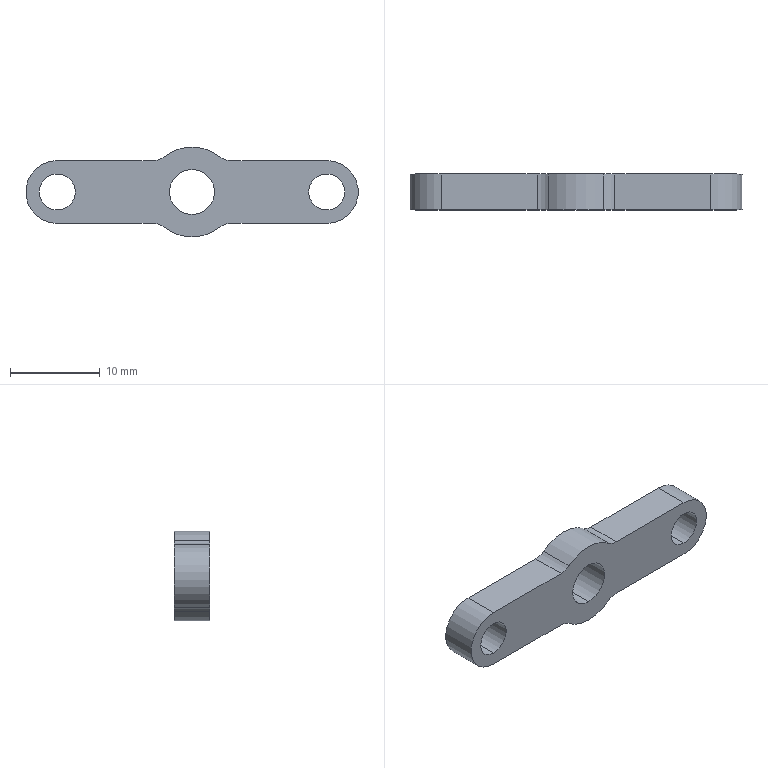Part | SolidWorks | features Extrusion 1, Scale 1 | 1 solid | 21 faces | box 37 x 4 x 10 mm | volume 874.953 mm3 | cylinder 15 | plane 6 | commonest cylinder face diameters 4 x8 10 x3 5 x2 7 x2
STEP:
#1=CARTESIAN_POINT('',(-15.,4.,-2.));
#2=VERTEX_POINT('',#1);
#3=CARTESIAN_POINT('',(-15.,4.,2.));
#4=VERTEX_POINT('',#3);
#5=CARTESIAN_POINT('',(-15.,4.,0.));
#6=DIRECTION('',(0.,1.,0.));
#7=DIRECTION('',(0.,0.,-1.));
#8=AXIS2_PLACEMENT_3D('',#5,#6,#7);
#9=CIRCLE('',#8,2.);
#10=EDGE_CURVE('',#2,#4,#9,.T.);
#11=ORIENTED_EDGE('',*,*,#10,.T.);
#12=CARTESIAN_POINT('',(-15.,0.,2.));
#13=VERTEX_POINT('',#12);
#14=CARTESIAN_POINT('',(-15.,4.,2.));
#15=DIRECTION('',(0.,-1.,0.));
#16=VECTOR('',#15,1000.);
#17=LINE('',#14,#16);
#18=EDGE_CURVE('',#4,#13,#17,.T.);
#19=ORIENTED_EDGE('',*,*,#18,.T.);
#20=CARTESIAN_POINT('',(-15.,0.,-2.));
#21=VERTEX_POINT('',#20);
#22=CARTESIAN_POINT('',(-15.,0.,0.));
#23=DIRECTION('',(0.,1.,0.));
#24=DIRECTION('',(0.,0.,-1.));
#25=AXIS2_PLACEMENT_3D('',#22,#23,#24);
#26=CIRCLE('',#25,2.);
#27=EDGE_CURVE('',#21,#13,#26,.T.);
#28=ORIENTED_EDGE('',*,*,#27,.F.);
#29=CARTESIAN_POINT('',(-15.,4.,-2.));
#30=DIRECTION('',(0.,-1.,0.));
#31=VECTOR('',#30,1000.);
#32=LINE('',#29,#31);
#33=EDGE_CURVE('',#2,#21,#32,.T.);
#34=ORIENTED_EDGE('',*,*,#33,.F.);
#35=EDGE_LOOP('',(#11,#19,#28,#34));
#36=FACE_OUTER_BOUND('',#35,.T.);
#37=CARTESIAN_POINT('',(-15.,4.,0.));
#38=DIRECTION('',(0.,-1.,0.));
#39=DIRECTION('',(0.,0.,-1.));
#40=AXIS2_PLACEMENT_3D('',#37,#38,#39);
#41=CYLINDRICAL_SURFACE('',#40,2.);
#42=ADVANCED_FACE('',(#36),#41,.F.);
#43=CARTESIAN_POINT('',(15.,4.,-2.));
#44=VERTEX_POINT('',#43);
#45=CARTESIAN_POINT('',(15.,4.,2.));
#46=VERTEX_POINT('',#45);
#47=CARTESIAN_POINT('',(15.,4.,0.));
#48=DIRECTION('',(0.,1.,0.));
#49=DIRECTION('',(0.,0.,1.));
#50=AXIS2_PLACEMENT_3D('',#47,#48,#49);
#51=CIRCLE('',#50,2.);
#52=EDGE_CURVE('',#44,#46,#51,.T.);
#53=ORIENTED_EDGE('',*,*,#52,.T.);
#54=CARTESIAN_POINT('',(15.,0.,2.));
#55=VERTEX_POINT('',#54);
#56=CARTESIAN_POINT('',(15.,4.,2.));
#57=DIRECTION('',(0.,-1.,0.));
#58=VECTOR('',#57,1000.);
#59=LINE('',#56,#58);
#60=EDGE_CURVE('',#46,#55,#59,.T.);
#61=ORIENTED_EDGE('',*,*,#60,.T.);
#62=CARTESIAN_POINT('',(15.,0.,-2.));
#63=VERTEX_POINT('',#62);
#64=CARTESIAN_POINT('',(15.,0.,0.));
#65=DIRECTION('',(0.,1.,0.));
#66=DIRECTION('',(0.,0.,1.));
#67=AXIS2_PLACEMENT_3D('',#64,#65,#66);
#68=CIRCLE('',#67,2.);
#69=EDGE_CURVE('',#63,#55,#68,.T.);
#70=ORIENTED_EDGE('',*,*,#69,.F.);
#71=CARTESIAN_POINT('',(15.,4.,-2.));
#72=DIRECTION('',(0.,-1.,0.));
#73=VECTOR('',#72,1000.);
#74=LINE('',#71,#73);
#75=EDGE_CURVE('',#44,#63,#74,.T.);
#76=ORIENTED_EDGE('',*,*,#75,.F.);
#77=EDGE_LOOP('',(#53,#61,#70,#76));
#78=FACE_OUTER_BOUND('',#77,.T.);
#79=CARTESIAN_POINT('',(15.,4.,0.));
#80=DIRECTION('',(0.,-1.,0.));
#81=DIRECTION('',(0.,0.,-1.));
#82=AXIS2_PLACEMENT_3D('',#79,#80,#81);
#83=CYLINDRICAL_SURFACE('',#82,2.);
#84=ADVANCED_FACE('',(#78),#83,.F.);
#85=CARTESIAN_POINT('',(0.,4.,-2.5));
#86=VERTEX_POINT('',#85);
#87=CARTESIAN_POINT('',(0.,4.,2.5));
#88=VERTEX_POINT('',#87);
#89=CARTESIAN_POINT('',(0.,4.,0.));
#90=DIRECTION('',(0.,1.,0.));
#91=DIRECTION('',(0.,0.,1.));
#92=AXIS2_PLACEMENT_3D('',#89,#90,#91);
#93=CIRCLE('',#92,2.5);
#94=EDGE_CURVE('',#86,#88,#93,.T.);
#95=ORIENTED_EDGE('',*,*,#94,.T.);
#96=CARTESIAN_POINT('',(0.,0.,2.5));
#97=VERTEX_POINT('',#96);
#98=CARTESIAN_POINT('',(0.,4.,2.5));
#99=DIRECTION('',(0.,-1.,0.));
#100=VECTOR('',#99,1000.);
#101=LINE('',#98,#100);
#102=EDGE_CURVE('',#88,#97,#101,.T.);
#103=ORIENTED_EDGE('',*,*,#102,.T.);
#104=CARTESIAN_POINT('',(0.,0.,-2.5));
#105=VERTEX_POINT('',#104);
#106=CARTESIAN_POINT('',(0.,0.,0.));
#107=DIRECTION('',(0.,1.,0.));
#108=DIRECTION('',(0.,0.,1.));
#109=AXIS2_PLACEMENT_3D('',#106,#107,#108);
#110=CIRCLE('',#109,2.5);
#111=EDGE_CURVE('',#105,#97,#110,.T.);
#112=ORIENTED_EDGE('',*,*,#111,.F.);
#113=CARTESIAN_POINT('',(0.,4.,-2.5));
#114=DIRECTION('',(0.,-1.,0.));
#115=VECTOR('',#114,1000.);
#116=LINE('',#113,#115);
#117=EDGE_CURVE('',#86,#105,#116,.T.);
#118=ORIENTED_EDGE('',*,*,#117,.F.);
#119=EDGE_LOOP('',(#95,#103,#112,#118));
#120=FACE_OUTER_BOUND('',#119,.T.);
#121=CARTESIAN_POINT('',(0.,4.,0.));
#122=DIRECTION('',(0.,-1.,0.));
#123=DIRECTION('',(0.,0.,-1.));
#124=AXIS2_PLACEMENT_3D('',#121,#122,#123);
#125=CYLINDRICAL_SURFACE('',#124,2.5);
#126=ADVANCED_FACE('',(#120),#125,.F.);
#127=CARTESIAN_POINT('',(0.,4.,-5.));
#128=VERTEX_POINT('',#127);
#129=CARTESIAN_POINT('',(-3.093,4.,-3.929));
#130=VERTEX_POINT('',#129);
#131=CARTESIAN_POINT('',(0.,4.,0.));
#132=DIRECTION('',(0.,1.,0.));
#133=DIRECTION('',(0.,0.,1.));
#134=AXIS2_PLACEMENT_3D('',#131,#132,#133);
#135=CIRCLE('',#134,5.);
#136=EDGE_CURVE('',#128,#130,#135,.T.);
#137=ORIENTED_EDGE('',*,*,#136,.F.);
#138=CARTESIAN_POINT('',(0.,0.,-5.));
#139=VERTEX_POINT('',#138);
#140=CARTESIAN_POINT('',(0.,4.,-5.));
#141=DIRECTION('',(0.,-1.,0.));
#142=VECTOR('',#141,1000.);
#143=LINE('',#140,#142);
#144=EDGE_CURVE('',#128,#139,#143,.T.);
#145=ORIENTED_EDGE('',*,*,#144,.T.);
#146=CARTESIAN_POINT('',(-3.093,0.,-3.929));
#147=VERTEX_POINT('',#146);
#148=CARTESIAN_POINT('',(0.,0.,0.));
#149=DIRECTION('',(0.,1.,0.));
#150=DIRECTION('',(0.,0.,1.));
#151=AXIS2_PLACEMENT_3D('',#148,#149,#150);
#152=CIRCLE('',#151,5.);
#153=EDGE_CURVE('',#139,#147,#152,.T.);
#154=ORIENTED_EDGE('',*,*,#153,.T.);
#155=CARTESIAN_POINT('',(-3.093,4.,-3.929));
#156=DIRECTION('',(0.,-1.,0.));
#157=VECTOR('',#156,1000.);
#158=LINE('',#155,#157);
#159=EDGE_CURVE('',#130,#147,#158,.T.);
#160=ORIENTED_EDGE('',*,*,#159,.F.);
#161=EDGE_LOOP('',(#137,#145,#154,#160));
#162=FACE_OUTER_BOUND('',#161,.T.);
#163=CARTESIAN_POINT('',(0.,4.,0.));
#164=DIRECTION('',(0.,-1.,0.));
#165=DIRECTION('',(0.,0.,-1.));
#166=AXIS2_PLACEMENT_3D('',#163,#164,#165);
#167=CYLINDRICAL_SURFACE('',#166,5.);
#168=ADVANCED_FACE('',(#162),#167,.T.);
#169=ORIENTED_EDGE('',*,*,#52,.F.);
#170=CARTESIAN_POINT('',(15.,4.,0.));
#171=DIRECTION('',(0.,1.,0.));
#172=DIRECTION('',(0.,0.,1.));
#173=AXIS2_PLACEMENT_3D('',#170,#171,#172);
#174=CIRCLE('',#173,2.);
#175=EDGE_CURVE('',#46,#44,#174,.T.);
#176=ORIENTED_EDGE('',*,*,#175,.F.);
#177=EDGE_LOOP('',(#169,#176));
#178=FACE_BOUND('',#177,.T.);
#179=CARTESIAN_POINT('',(3.093,4.,3.929));
#180=VERTEX_POINT('',#179);
#181=CARTESIAN_POINT('',(4.33,4.,3.5));
#182=VERTEX_POINT('',#181);
#183=CARTESIAN_POINT('',(4.33,4.,5.5));
#184=DIRECTION('',(0.,-1.,0.));
#185=DIRECTION('',(0.,0.,1.));
#186=AXIS2_PLACEMENT_3D('',#183,#184,#185);
#187=CIRCLE('',#186,2.);
#188=EDGE_CURVE('',#180,#182,#187,.T.);
#189=ORIENTED_EDGE('',*,*,#188,.T.);
#190=CARTESIAN_POINT('',(15.,4.,3.5));
#191=VERTEX_POINT('',#190);
#192=CARTESIAN_POINT('',(15.,4.,3.5));
#193=DIRECTION('',(1.,0.,0.));
#194=VECTOR('',#193,1000.);
#195=LINE('',#192,#194);
#196=EDGE_CURVE('',#182,#191,#195,.T.);
#197=ORIENTED_EDGE('',*,*,#196,.T.);
#198=CARTESIAN_POINT('',(15.,4.,-3.5));
#199=VERTEX_POINT('',#198);
#200=CARTESIAN_POINT('',(15.,4.,0.));
#201=DIRECTION('',(0.,1.,0.));
#202=DIRECTION('',(0.,0.,1.));
#203=AXIS2_PLACEMENT_3D('',#200,#201,#202);
#204=CIRCLE('',#203,3.5);
#205=EDGE_CURVE('',#191,#199,#204,.T.);
#206=ORIENTED_EDGE('',*,*,#205,.T.);
#207=CARTESIAN_POINT('',(4.33,4.,-3.5));
#208=VERTEX_POINT('',#207);
#209=CARTESIAN_POINT('',(15.,4.,-3.5));
#210=DIRECTION('',(-1.,0.,0.));
#211=VECTOR('',#210,1000.);
#212=LINE('',#209,#211);
#213=EDGE_CURVE('',#199,#208,#212,.T.);
#214=ORIENTED_EDGE('',*,*,#213,.T.);
#215=CARTESIAN_POINT('',(3.093,4.,-3.929));
#216=VERTEX_POINT('',#215);
#217=CARTESIAN_POINT('',(4.33,4.,-5.5));
#218=DIRECTION('',(0.,-1.,0.));
#219=DIRECTION('',(0.,0.,-1.));
#220=AXIS2_PLACEMENT_3D('',#217,#218,#219);
#221=CIRCLE('',#220,2.);
#222=EDGE_CURVE('',#208,#216,#221,.T.);
#223=ORIENTED_EDGE('',*,*,#222,.T.);
#224=CARTESIAN_POINT('',(0.,4.,0.));
#225=DIRECTION('',(0.,1.,0.));
#226=DIRECTION('',(0.,0.,1.));
#227=AXIS2_PLACEMENT_3D('',#224,#225,#226);
#228=CIRCLE('',#227,5.);
#229=EDGE_CURVE('',#216,#128,#228,.T.);
#230=ORIENTED_EDGE('',*,*,#229,.T.);
#231=ORIENTED_EDGE('',*,*,#136,.T.);
#232=CARTESIAN_POINT('',(-4.33,4.,-3.5));
#233=VERTEX_POINT('',#232);
#234=CARTESIAN_POINT('',(-4.33,4.,-5.5));
#235=DIRECTION('',(0.,-1.,0.));
#236=DIRECTION('',(0.,0.,1.));
#237=AXIS2_PLACEMENT_3D('',#234,#235,#236);
#238=CIRCLE('',#237,2.);
#239=EDGE_CURVE('',#130,#233,#238,.T.);
#240=ORIENTED_EDGE('',*,*,#239,.T.);
#241=CARTESIAN_POINT('',(-15.,4.,-3.5));
#242=VERTEX_POINT('',#241);
#243=CARTESIAN_POINT('',(-15.,4.,-3.5));
#244=DIRECTION('',(-1.,0.,0.));
#245=VECTOR('',#244,1000.);
#246=LINE('',#243,#245);
#247=EDGE_CURVE('',#233,#242,#246,.T.);
#248=ORIENTED_EDGE('',*,*,#247,.T.);
#249=CARTESIAN_POINT('',(-15.,4.,3.5));
#250=VERTEX_POINT('',#249);
#251=CARTESIAN_POINT('',(-15.,4.,0.));
#252=DIRECTION('',(0.,1.,0.));
#253=DIRECTION('',(0.,0.,-1.));
#254=AXIS2_PLACEMENT_3D('',#251,#252,#253);
#255=CIRCLE('',#254,3.5);
#256=EDGE_CURVE('',#242,#250,#255,.T.);
#257=ORIENTED_EDGE('',*,*,#256,.T.);
#258=CARTESIAN_POINT('',(-4.33,4.,3.5));
#259=VERTEX_POINT('',#258);
#260=CARTESIAN_POINT('',(-15.,4.,3.5));
#261=DIRECTION('',(1.,0.,0.));
#262=VECTOR('',#261,1000.);
#263=LINE('',#260,#262);
#264=EDGE_CURVE('',#250,#259,#263,.T.);
#265=ORIENTED_EDGE('',*,*,#264,.T.);
#266=CARTESIAN_POINT('',(-3.093,4.,3.929));
#267=VERTEX_POINT('',#266);
#268=CARTESIAN_POINT('',(-4.33,4.,5.5));
#269=DIRECTION('',(0.,-1.,0.));
#270=DIRECTION('',(0.,0.,-1.));
#271=AXIS2_PLACEMENT_3D('',#268,#269,#270);
#272=CIRCLE('',#271,2.);
#273=EDGE_CURVE('',#259,#267,#272,.T.);
#274=ORIENTED_EDGE('',*,*,#273,.T.);
#275=CARTESIAN_POINT('',(0.,4.,0.));
#276=DIRECTION('',(0.,1.,0.));
#277=DIRECTION('',(0.,0.,1.));
#278=AXIS2_PLACEMENT_3D('',#275,#276,#277);
#279=CIRCLE('',#278,5.);
#280=EDGE_CURVE('',#267,#180,#279,.T.);
#281=ORIENTED_EDGE('',*,*,#280,.T.);
#282=EDGE_LOOP('',(#189,#197,#206,#214,#223,#230,#231,#240,#248,#257,#265,#274,#281));
#283=FACE_OUTER_BOUND('',#282,.T.);
#284=ORIENTED_EDGE('',*,*,#94,.F.);
#285=CARTESIAN_POINT('',(0.,4.,0.));
#286=DIRECTION('',(0.,1.,0.));
#287=DIRECTION('',(0.,0.,1.));
#288=AXIS2_PLACEMENT_3D('',#285,#286,#287);
#289=CIRCLE('',#288,2.5);
#290=EDGE_CURVE('',#88,#86,#289,.T.);
#291=ORIENTED_EDGE('',*,*,#290,.F.);
#292=EDGE_LOOP('',(#284,#291));
#293=FACE_BOUND('',#292,.T.);
#294=ORIENTED_EDGE('',*,*,#10,.F.);
#295=CARTESIAN_POINT('',(-15.,4.,0.));
#296=DIRECTION('',(0.,1.,0.));
#297=DIRECTION('',(0.,0.,-1.));
#298=AXIS2_PLACEMENT_3D('',#295,#296,#297);
#299=CIRCLE('',#298,2.);
#300=EDGE_CURVE('',#4,#2,#299,.T.);
#301=ORIENTED_EDGE('',*,*,#300,.F.);
#302=EDGE_LOOP('',(#294,#301));
#303=FACE_BOUND('',#302,.T.);
#304=CARTESIAN_POINT('',(4.33,4.,5.5));
#305=DIRECTION('',(0.,1.,0.));
#306=DIRECTION('',(0.,0.,1.));
#307=AXIS2_PLACEMENT_3D('',#304,#305,#306);
#308=PLANE('',#307);
#309=ADVANCED_FACE('',(#178,#283,#293,#303),#308,.T.);
#310=CARTESIAN_POINT('',(3.093,0.,3.929));
#311=VERTEX_POINT('',#310);
#312=CARTESIAN_POINT('',(4.33,0.,3.5));
#313=VERTEX_POINT('',#312);
#314=CARTESIAN_POINT('',(4.33,0.,5.5));
#315=DIRECTION('',(0.,-1.,0.));
#316=DIRECTION('',(0.,0.,1.));
#317=AXIS2_PLACEMENT_3D('',#314,#315,#316);
#318=CIRCLE('',#317,2.);
#319=EDGE_CURVE('',#311,#313,#318,.T.);
#320=ORIENTED_EDGE('',*,*,#319,.F.);
#321=CARTESIAN_POINT('',(-3.093,0.,3.929));
#322=VERTEX_POINT('',#321);
#323=CARTESIAN_POINT('',(0.,0.,0.));
#324=DIRECTION('',(0.,1.,0.));
#325=DIRECTION('',(0.,0.,1.));
#326=AXIS2_PLACEMENT_3D('',#323,#324,#325);
#327=CIRCLE('',#326,5.);
#328=EDGE_CURVE('',#322,#311,#327,.T.);
#329=ORIENTED_EDGE('',*,*,#328,.F.);
#330=CARTESIAN_POINT('',(-4.33,0.,3.5));
#331=VERTEX_POINT('',#330);
#332=CARTESIAN_POINT('',(-4.33,0.,5.5));
#333=DIRECTION('',(0.,-1.,0.));
#334=DIRECTION('',(0.,0.,-1.));
#335=AXIS2_PLACEMENT_3D('',#332,#333,#334);
#336=CIRCLE('',#335,2.);
#337=EDGE_CURVE('',#331,#322,#336,.T.);
#338=ORIENTED_EDGE('',*,*,#337,.F.);
#339=CARTESIAN_POINT('',(-15.,0.,3.5));
#340=VERTEX_POINT('',#339);
#341=CARTESIAN_POINT('',(-15.,0.,3.5));
#342=DIRECTION('',(1.,0.,0.));
#343=VECTOR('',#342,1000.);
#344=LINE('',#341,#343);
#345=EDGE_CURVE('',#340,#331,#344,.T.);
#346=ORIENTED_EDGE('',*,*,#345,.F.);
#347=CARTESIAN_POINT('',(-15.,0.,-3.5));
#348=VERTEX_POINT('',#347);
#349=CARTESIAN_POINT('',(-15.,0.,0.));
#350=DIRECTION('',(0.,1.,0.));
#351=DIRECTION('',(0.,0.,-1.));
#352=AXIS2_PLACEMENT_3D('',#349,#350,#351);
#353=CIRCLE('',#352,3.5);
#354=EDGE_CURVE('',#348,#340,#353,.T.);
#355=ORIENTED_EDGE('',*,*,#354,.F.);
#356=CARTESIAN_POINT('',(-4.33,0.,-3.5));
#357=VERTEX_POINT('',#356);
#358=CARTESIAN_POINT('',(-15.,0.,-3.5));
#359=DIRECTION('',(-1.,0.,0.));
#360=VECTOR('',#359,1000.);
#361=LINE('',#358,#360);
#362=EDGE_CURVE('',#357,#348,#361,.T.);
#363=ORIENTED_EDGE('',*,*,#362,.F.);
#364=CARTESIAN_POINT('',(-4.33,0.,-5.5));
#365=DIRECTION('',(0.,-1.,0.));
#366=DIRECTION('',(0.,0.,1.));
#367=AXIS2_PLACEMENT_3D('',#364,#365,#366);
#368=CIRCLE('',#367,2.);
#369=EDGE_CURVE('',#147,#357,#368,.T.);
#370=ORIENTED_EDGE('',*,*,#369,.F.);
#371=ORIENTED_EDGE('',*,*,#153,.F.);
#372=CARTESIAN_POINT('',(3.093,0.,-3.929));
#373=VERTEX_POINT('',#372);
#374=CARTESIAN_POINT('',(0.,0.,0.));
#375=DIRECTION('',(0.,1.,0.));
#376=DIRECTION('',(0.,0.,1.));
#377=AXIS2_PLACEMENT_3D('',#374,#375,#376);
#378=CIRCLE('',#377,5.);
#379=EDGE_CURVE('',#373,#139,#378,.T.);
#380=ORIENTED_EDGE('',*,*,#379,.F.);
#381=CARTESIAN_POINT('',(4.33,0.,-3.5));
#382=VERTEX_POINT('',#381);
#383=CARTESIAN_POINT('',(4.33,0.,-5.5));
#384=DIRECTION('',(0.,-1.,0.));
#385=DIRECTION('',(0.,0.,-1.));
#386=AXIS2_PLACEMENT_3D('',#383,#384,#385);
#387=CIRCLE('',#386,2.);
#388=EDGE_CURVE('',#382,#373,#387,.T.);
#389=ORIENTED_EDGE('',*,*,#388,.F.);
#390=CARTESIAN_POINT('',(15.,0.,-3.5));
#391=VERTEX_POINT('',#390);
#392=CARTESIAN_POINT('',(15.,0.,-3.5));
#393=DIRECTION('',(-1.,0.,0.));
#394=VECTOR('',#393,1000.);
#395=LINE('',#392,#394);
#396=EDGE_CURVE('',#391,#382,#395,.T.);
#397=ORIENTED_EDGE('',*,*,#396,.F.);
#398=CARTESIAN_POINT('',(15.,0.,3.5));
#399=VERTEX_POINT('',#398);
#400=CARTESIAN_POINT('',(15.,0.,0.));
#401=DIRECTION('',(0.,1.,0.));
#402=DIRECTION('',(0.,0.,1.));
#403=AXIS2_PLACEMENT_3D('',#400,#401,#402);
#404=CIRCLE('',#403,3.5);
#405=EDGE_CURVE('',#399,#391,#404,.T.);
#406=ORIENTED_EDGE('',*,*,#405,.F.);
#407=CARTESIAN_POINT('',(15.,0.,3.5));
#408=DIRECTION('',(1.,0.,0.));
#409=VECTOR('',#408,1000.);
#410=LINE('',#407,#409);
#411=EDGE_CURVE('',#313,#399,#410,.T.);
#412=ORIENTED_EDGE('',*,*,#411,.F.);
#413=EDGE_LOOP('',(#320,#329,#338,#346,#355,#363,#370,#371,#380,#389,#397,#406,#412));
#414=FACE_OUTER_BOUND('',#413,.T.);
#415=ORIENTED_EDGE('',*,*,#111,.T.);
#416=CARTESIAN_POINT('',(0.,0.,0.));
#417=DIRECTION('',(0.,1.,0.));
#418=DIRECTION('',(0.,0.,1.));
#419=AXIS2_PLACEMENT_3D('',#416,#417,#418);
#420=CIRCLE('',#419,2.5);
#421=EDGE_CURVE('',#97,#105,#420,.T.);
#422=ORIENTED_EDGE('',*,*,#421,.T.);
#423=EDGE_LOOP('',(#415,#422));
#424=FACE_BOUND('',#423,.T.);
#425=ORIENTED_EDGE('',*,*,#69,.T.);
#426=CARTESIAN_POINT('',(15.,0.,0.));
#427=DIRECTION('',(0.,1.,0.));
#428=DIRECTION('',(0.,0.,1.));
#429=AXIS2_PLACEMENT_3D('',#426,#427,#428);
#430=CIRCLE('',#429,2.);
#431=EDGE_CURVE('',#55,#63,#430,.T.);
#432=ORIENTED_EDGE('',*,*,#431,.T.);
#433=EDGE_LOOP('',(#425,#432));
#434=FACE_BOUND('',#433,.T.);
#435=ORIENTED_EDGE('',*,*,#27,.T.);
#436=CARTESIAN_POINT('',(-15.,0.,0.));
#437=DIRECTION('',(0.,1.,0.));
#438=DIRECTION('',(0.,0.,-1.));
#439=AXIS2_PLACEMENT_3D('',#436,#437,#438);
#440=CIRCLE('',#439,2.);
#441=EDGE_CURVE('',#13,#21,#440,.T.);
#442=ORIENTED_EDGE('',*,*,#441,.T.);
#443=EDGE_LOOP('',(#435,#442));
#444=FACE_BOUND('',#443,.T.);
#445=CARTESIAN_POINT('',(4.33,0.,5.5));
#446=DIRECTION('',(0.,1.,0.));
#447=DIRECTION('',(0.,0.,1.));
#448=AXIS2_PLACEMENT_3D('',#445,#446,#447);
#449=PLANE('',#448);
#450=ADVANCED_FACE('',(#414,#424,#434,#444),#449,.F.);
#451=ORIENTED_EDGE('',*,*,#319,.T.);
#452=CARTESIAN_POINT('',(4.33,4.,3.5));
#453=DIRECTION('',(0.,-1.,0.));
#454=VECTOR('',#453,1000.);
#455=LINE('',#452,#454);
#456=EDGE_CURVE('',#182,#313,#455,.T.);
#457=ORIENTED_EDGE('',*,*,#456,.F.);
#458=ORIENTED_EDGE('',*,*,#188,.F.);
#459=CARTESIAN_POINT('',(3.093,4.,3.929));
#460=DIRECTION('',(0.,-1.,0.));
#461=VECTOR('',#460,1000.);
#462=LINE('',#459,#461);
#463=EDGE_CURVE('',#180,#311,#462,.T.);
#464=ORIENTED_EDGE('',*,*,#463,.T.);
#465=EDGE_LOOP('',(#451,#457,#458,#464));
#466=FACE_OUTER_BOUND('',#465,.T.);
#467=CARTESIAN_POINT('',(4.33,4.,5.5));
#468=DIRECTION('',(0.,-1.,0.));
#469=DIRECTION('',(0.,0.,-1.));
#470=AXIS2_PLACEMENT_3D('',#467,#468,#469);
#471=CYLINDRICAL_SURFACE('',#470,2.);
#472=ADVANCED_FACE('',(#466),#471,.F.);
#473=ORIENTED_EDGE('',*,*,#411,.T.);
#474=CARTESIAN_POINT('',(15.,4.,3.5));
#475=DIRECTION('',(0.,-1.,0.));
#476=VECTOR('',#475,1000.);
#477=LINE('',#474,#476);
#478=EDGE_CURVE('',#191,#399,#477,.T.);
#479=ORIENTED_EDGE('',*,*,#478,.F.);
#480=ORIENTED_EDGE('',*,*,#196,.F.);
#481=ORIENTED_EDGE('',*,*,#456,.T.);
#482=EDGE_LOOP('',(#473,#479,#480,#481));
#483=FACE_OUTER_BOUND('',#482,.T.);
#484=CARTESIAN_POINT('',(15.,4.,3.5));
#485=DIRECTION('',(0.,0.,-1.));
#486=DIRECTION('',(-1.,0.,0.));
#487=AXIS2_PLACEMENT_3D('',#484,#485,#486);
#488=PLANE('',#487);
#489=ADVANCED_FACE('',(#483),#488,.F.);
#490=ORIENTED_EDGE('',*,*,#405,.T.);
#491=CARTESIAN_POINT('',(15.,4.,-3.5));
#492=DIRECTION('',(0.,-1.,0.));
#493=VECTOR('',#492,1000.);
#494=LINE('',#491,#493);
#495=EDGE_CURVE('',#199,#391,#494,.T.);
#496=ORIENTED_EDGE('',*,*,#495,.F.);
#497=ORIENTED_EDGE('',*,*,#205,.F.);
#498=ORIENTED_EDGE('',*,*,#478,.T.);
#499=EDGE_LOOP('',(#490,#496,#497,#498));
#500=FACE_OUTER_BOUND('',#499,.T.);
#501=CARTESIAN_POINT('',(15.,4.,0.));
#502=DIRECTION('',(0.,-1.,0.));
#503=DIRECTION('',(0.,0.,-1.));
#504=AXIS2_PLACEMENT_3D('',#501,#502,#503);
#505=CYLINDRICAL_SURFACE('',#504,3.5);
#506=ADVANCED_FACE('',(#500),#505,.T.);
#507=ORIENTED_EDGE('',*,*,#396,.T.);
#508=CARTESIAN_POINT('',(4.33,4.,-3.5));
#509=DIRECTION('',(0.,-1.,0.));
#510=VECTOR('',#509,1000.);
#511=LINE('',#508,#510);
#512=EDGE_CURVE('',#208,#382,#511,.T.);
#513=ORIENTED_EDGE('',*,*,#512,.F.);
#514=ORIENTED_EDGE('',*,*,#213,.F.);
#515=ORIENTED_EDGE('',*,*,#495,.T.);
#516=EDGE_LOOP('',(#507,#513,#514,#515));
#517=FACE_OUTER_BOUND('',#516,.T.);
#518=CARTESIAN_POINT('',(15.,4.,-3.5));
#519=DIRECTION('',(0.,0.,1.));
#520=DIRECTION('',(1.,0.,0.));
#521=AXIS2_PLACEMENT_3D('',#518,#519,#520);
#522=PLANE('',#521);
#523=ADVANCED_FACE('',(#517),#522,.F.);
#524=ORIENTED_EDGE('',*,*,#388,.T.);
#525=CARTESIAN_POINT('',(3.093,4.,-3.929));
#526=DIRECTION('',(0.,-1.,0.));
#527=VECTOR('',#526,1000.);
#528=LINE('',#525,#527);
#529=EDGE_CURVE('',#216,#373,#528,.T.);
#530=ORIENTED_EDGE('',*,*,#529,.F.);
#531=ORIENTED_EDGE('',*,*,#222,.F.);
#532=ORIENTED_EDGE('',*,*,#512,.T.);
#533=EDGE_LOOP('',(#524,#530,#531,#532));
#534=FACE_OUTER_BOUND('',#533,.T.);
#535=CARTESIAN_POINT('',(4.33,4.,-5.5));
#536=DIRECTION('',(0.,-1.,0.));
#537=DIRECTION('',(0.,0.,-1.));
#538=AXIS2_PLACEMENT_3D('',#535,#536,#537);
#539=CYLINDRICAL_SURFACE('',#538,2.);
#540=ADVANCED_FACE('',(#534),#539,.F.);
#541=ORIENTED_EDGE('',*,*,#144,.F.);
#542=ORIENTED_EDGE('',*,*,#229,.F.);
#543=ORIENTED_EDGE('',*,*,#529,.T.);
#544=ORIENTED_EDGE('',*,*,#379,.T.);
#545=EDGE_LOOP('',(#541,#542,#543,#544));
#546=FACE_OUTER_BOUND('',#545,.T.);
#547=CARTESIAN_POINT('',(0.,4.,0.));
#548=DIRECTION('',(0.,-1.,0.));
#549=DIRECTION('',(0.,0.,-1.));
#550=AXIS2_PLACEMENT_3D('',#547,#548,#549);
#551=CYLINDRICAL_SURFACE('',#550,5.);
#552=ADVANCED_FACE('',(#546),#551,.T.);
#553=ORIENTED_EDGE('',*,*,#369,.T.);
#554=CARTESIAN_POINT('',(-4.33,4.,-3.5));
#555=DIRECTION('',(0.,-1.,0.));
#556=VECTOR('',#555,1000.);
#557=LINE('',#554,#556);
#558=EDGE_CURVE('',#233,#357,#557,.T.);
#559=ORIENTED_EDGE('',*,*,#558,.F.);
#560=ORIENTED_EDGE('',*,*,#239,.F.);
#561=ORIENTED_EDGE('',*,*,#159,.T.);
#562=EDGE_LOOP('',(#553,#559,#560,#561));
#563=FACE_OUTER_BOUND('',#562,.T.);
#564=CARTESIAN_POINT('',(-4.33,4.,-5.5));
#565=DIRECTION('',(0.,-1.,0.));
#566=DIRECTION('',(0.,0.,-1.));
#567=AXIS2_PLACEMENT_3D('',#564,#565,#566);
#568=CYLINDRICAL_SURFACE('',#567,2.);
#569=ADVANCED_FACE('',(#563),#568,.F.);
#570=ORIENTED_EDGE('',*,*,#362,.T.);
#571=CARTESIAN_POINT('',(-15.,4.,-3.5));
#572=DIRECTION('',(0.,-1.,0.));
#573=VECTOR('',#572,1000.);
#574=LINE('',#571,#573);
#575=EDGE_CURVE('',#242,#348,#574,.T.);
#576=ORIENTED_EDGE('',*,*,#575,.F.);
#577=ORIENTED_EDGE('',*,*,#247,.F.);
#578=ORIENTED_EDGE('',*,*,#558,.T.);
#579=EDGE_LOOP('',(#570,#576,#577,#578));
#580=FACE_OUTER_BOUND('',#579,.T.);
#581=CARTESIAN_POINT('',(-15.,4.,-3.5));
#582=DIRECTION('',(0.,0.,1.));
#583=DIRECTION('',(1.,0.,0.));
#584=AXIS2_PLACEMENT_3D('',#581,#582,#583);
#585=PLANE('',#584);
#586=ADVANCED_FACE('',(#580),#585,.F.);
#587=ORIENTED_EDGE('',*,*,#354,.T.);
#588=CARTESIAN_POINT('',(-15.,4.,3.5));
#589=DIRECTION('',(0.,-1.,0.));
#590=VECTOR('',#589,1000.);
#591=LINE('',#588,#590);
#592=EDGE_CURVE('',#250,#340,#591,.T.);
#593=ORIENTED_EDGE('',*,*,#592,.F.);
#594=ORIENTED_EDGE('',*,*,#256,.F.);
#595=ORIENTED_EDGE('',*,*,#575,.T.);
#596=EDGE_LOOP('',(#587,#593,#594,#595));
#597=FACE_OUTER_BOUND('',#596,.T.);
#598=CARTESIAN_POINT('',(-15.,4.,0.));
#599=DIRECTION('',(0.,-1.,0.));
#600=DIRECTION('',(0.,0.,-1.));
#601=AXIS2_PLACEMENT_3D('',#598,#599,#600);
#602=CYLINDRICAL_SURFACE('',#601,3.5);
#603=ADVANCED_FACE('',(#597),#602,.T.);
#604=ORIENTED_EDGE('',*,*,#345,.T.);
#605=CARTESIAN_POINT('',(-4.33,4.,3.5));
#606=DIRECTION('',(0.,-1.,0.));
#607=VECTOR('',#606,1000.);
#608=LINE('',#605,#607);
#609=EDGE_CURVE('',#259,#331,#608,.T.);
#610=ORIENTED_EDGE('',*,*,#609,.F.);
#611=ORIENTED_EDGE('',*,*,#264,.F.);
#612=ORIENTED_EDGE('',*,*,#592,.T.);
#613=EDGE_LOOP('',(#604,#610,#611,#612));
#614=FACE_OUTER_BOUND('',#613,.T.);
#615=CARTESIAN_POINT('',(-15.,4.,3.5));
#616=DIRECTION('',(0.,0.,-1.));
#617=DIRECTION('',(-1.,0.,0.));
#618=AXIS2_PLACEMENT_3D('',#615,#616,#617);
#619=PLANE('',#618);
#620=ADVANCED_FACE('',(#614),#619,.F.);
#621=ORIENTED_EDGE('',*,*,#337,.T.);
#622=CARTESIAN_POINT('',(-3.093,4.,3.929));
#623=DIRECTION('',(0.,-1.,0.));
#624=VECTOR('',#623,1000.);
#625=LINE('',#622,#624);
#626=EDGE_CURVE('',#267,#322,#625,.T.);
#627=ORIENTED_EDGE('',*,*,#626,.F.);
#628=ORIENTED_EDGE('',*,*,#273,.F.);
#629=ORIENTED_EDGE('',*,*,#609,.T.);
#630=EDGE_LOOP('',(#621,#627,#628,#629));
#631=FACE_OUTER_BOUND('',#630,.T.);
#632=CARTESIAN_POINT('',(-4.33,4.,5.5));
#633=DIRECTION('',(0.,-1.,0.));
#634=DIRECTION('',(0.,0.,-1.));
#635=AXIS2_PLACEMENT_3D('',#632,#633,#634);
#636=CYLINDRICAL_SURFACE('',#635,2.);
#637=ADVANCED_FACE('',(#631),#636,.F.);
#638=ORIENTED_EDGE('',*,*,#328,.T.);
#639=ORIENTED_EDGE('',*,*,#463,.F.);
#640=ORIENTED_EDGE('',*,*,#280,.F.);
#641=ORIENTED_EDGE('',*,*,#626,.T.);
#642=EDGE_LOOP('',(#638,#639,#640,#641));
#643=FACE_OUTER_BOUND('',#642,.T.);
#644=CARTESIAN_POINT('',(0.,4.,0.));
#645=DIRECTION('',(0.,-1.,0.));
#646=DIRECTION('',(0.,0.,-1.));
#647=AXIS2_PLACEMENT_3D('',#644,#645,#646);
#648=CYLINDRICAL_SURFACE('',#647,5.);
#649=ADVANCED_FACE('',(#643),#648,.T.);
#650=ORIENTED_EDGE('',*,*,#102,.F.);
#651=ORIENTED_EDGE('',*,*,#290,.T.);
#652=ORIENTED_EDGE('',*,*,#117,.T.);
#653=ORIENTED_EDGE('',*,*,#421,.F.);
#654=EDGE_LOOP('',(#650,#651,#652,#653));
#655=FACE_OUTER_BOUND('',#654,.T.);
#656=CARTESIAN_POINT('',(0.,4.,0.));
#657=DIRECTION('',(0.,-1.,0.));
#658=DIRECTION('',(0.,0.,-1.));
#659=AXIS2_PLACEMENT_3D('',#656,#657,#658);
#660=CYLINDRICAL_SURFACE('',#659,2.5);
#661=ADVANCED_FACE('',(#655),#660,.F.);
#662=ORIENTED_EDGE('',*,*,#60,.F.);
#663=ORIENTED_EDGE('',*,*,#175,.T.);
#664=ORIENTED_EDGE('',*,*,#75,.T.);
#665=ORIENTED_EDGE('',*,*,#431,.F.);
#666=EDGE_LOOP('',(#662,#663,#664,#665));
#667=FACE_OUTER_BOUND('',#666,.T.);
#668=CARTESIAN_POINT('',(15.,4.,0.));
#669=DIRECTION('',(0.,-1.,0.));
#670=DIRECTION('',(0.,0.,-1.));
#671=AXIS2_PLACEMENT_3D('',#668,#669,#670);
#672=CYLINDRICAL_SURFACE('',#671,2.);
#673=ADVANCED_FACE('',(#667),#672,.F.);
#674=ORIENTED_EDGE('',*,*,#18,.F.);
#675=ORIENTED_EDGE('',*,*,#300,.T.);
#676=ORIENTED_EDGE('',*,*,#33,.T.);
#677=ORIENTED_EDGE('',*,*,#441,.F.);
#678=EDGE_LOOP('',(#674,#675,#676,#677));
#679=FACE_OUTER_BOUND('',#678,.T.);
#680=CARTESIAN_POINT('',(-15.,4.,0.));
#681=DIRECTION('',(0.,-1.,0.));
#682=DIRECTION('',(0.,0.,-1.));
#683=AXIS2_PLACEMENT_3D('',#680,#681,#682);
#684=CYLINDRICAL_SURFACE('',#683,2.);
#685=ADVANCED_FACE('',(#679),#684,.F.);
#686=CLOSED_SHELL('',(#42,#84,#126,#168,#309,#450,#472,#489,#506,#523,#540,#552,#569,#586,#603,#620,#637,#649,#661,#673,#685));
#687=MANIFOLD_SOLID_BREP('',#686);
#688=CARTESIAN_POINT('',(0.,0.,0.));
#689=DIRECTION('',(0.,0.,1.));
#690=DIRECTION('',(1.,0.,0.));
#691=AXIS2_PLACEMENT_3D('',#688,#689,#690);
#692=(LENGTH_UNIT()NAMED_UNIT(*)SI_UNIT(.MILLI.,.METRE.));
#693=UNCERTAINTY_MEASURE_WITH_UNIT(LENGTH_MEASURE(0.00001),#692,'','');
#694=(NAMED_UNIT(*)PLANE_ANGLE_UNIT()SI_UNIT($,.RADIAN.));
#695=(NAMED_UNIT(*)SI_UNIT($,.STERADIAN.)SOLID_ANGLE_UNIT());
#696=(GEOMETRIC_REPRESENTATION_CONTEXT(3)GLOBAL_UNCERTAINTY_ASSIGNED_CONTEXT((#693))GLOBAL_UNIT_ASSIGNED_CONTEXT((#692,#694,#695))REPRESENTATION_CONTEXT('',''));
#697=ADVANCED_BREP_SHAPE_REPRESENTATION('',(#687,#691),#696);